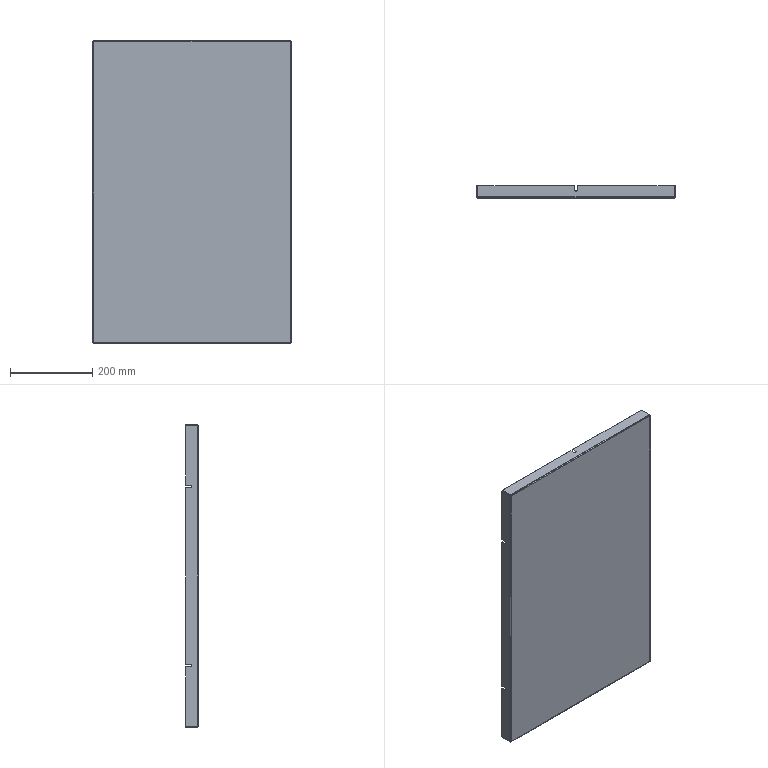Part | STEP file | JBJ-P-1000-12 | 1 solid | 62 faces | box 481 x 30 x 735 mm | volume 630028 mm3 | plane 40 | cylinder 14 | spline 8 | commonest cylinder face diameters 6.5 x6 2 x4 5 x4